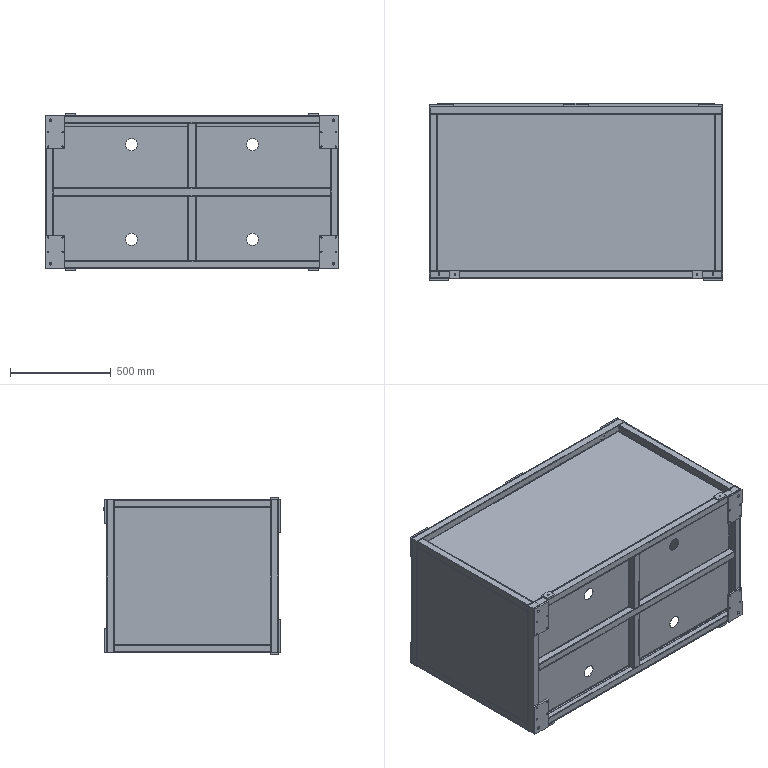Part | SolidWorks | features HoleWzd 6, ICE 5, FlatPattern 3, SMBaseFlange 3, SheetMetal 3, EdgeFlange 2, 3DProfileFeature 1, MirrorPattern 1, MoveFace 1, WeldMemberFeat 1, WeldmentFeature 1 | 31 solids | 618 faces | box 1453 x 880 x 780 mm | volume 27439038 mm3 | plane 312 | cylinder 284 | spline 16 | cone 6 | commonest cylinder face diameters 6.8 x88 4 x68 2 x64 14 x32 1 x8 2.5 x8